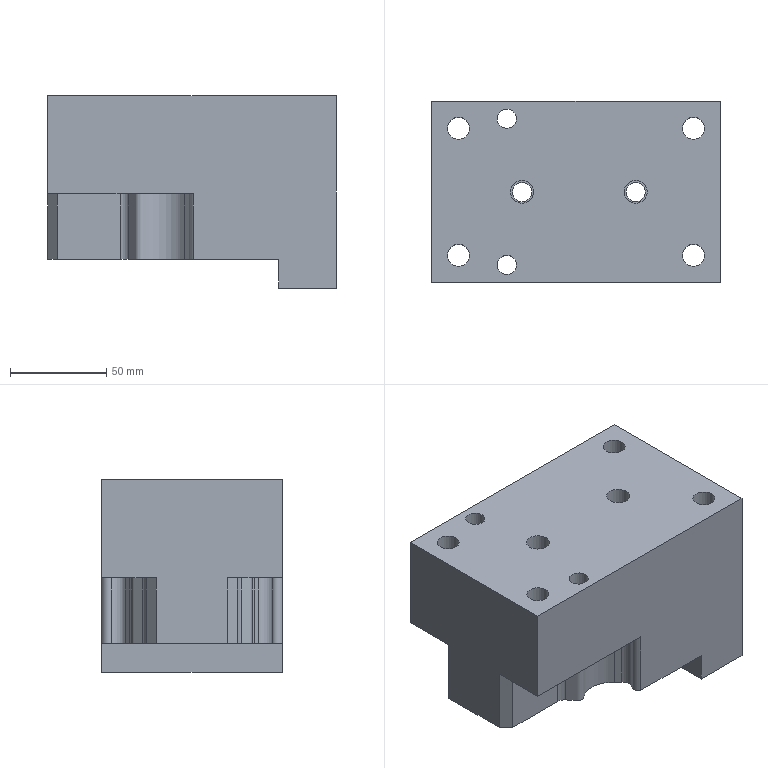Part | NX | features 7 2 | 1 solid | 60 faces | box 150 x 94 x 100 mm | volume 1042396 mm3 | cylinder 26 | plane 24 | cone 6 | spline 4 | commonest cylinder face diameters 8.5 x4 10 x4 10.001 x4 11.5 x4 18 x4 8.499 x2